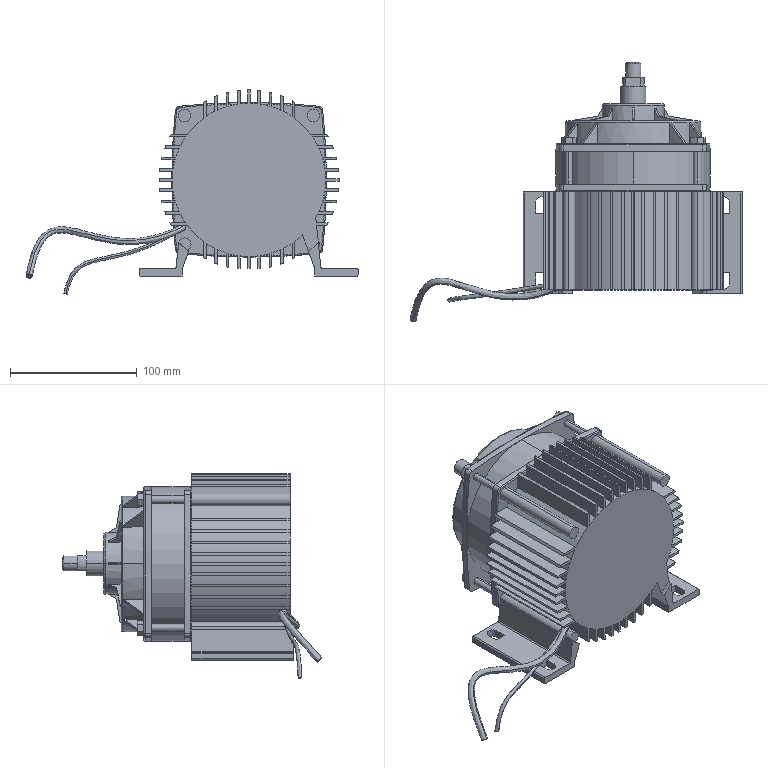Part | SolidWorks | features BaseBody 1 | 1 solid | 443 faces | box 262.331 x 205.132 x 161.422 mm | volume 1717621 mm3 | plane 267 | cylinder 127 | cone 22 | torus 22 | spline 5 | commonest cylinder face diameters 121 x36 142.263 x34 1067 x10 6 x8 7 x8 10 x8